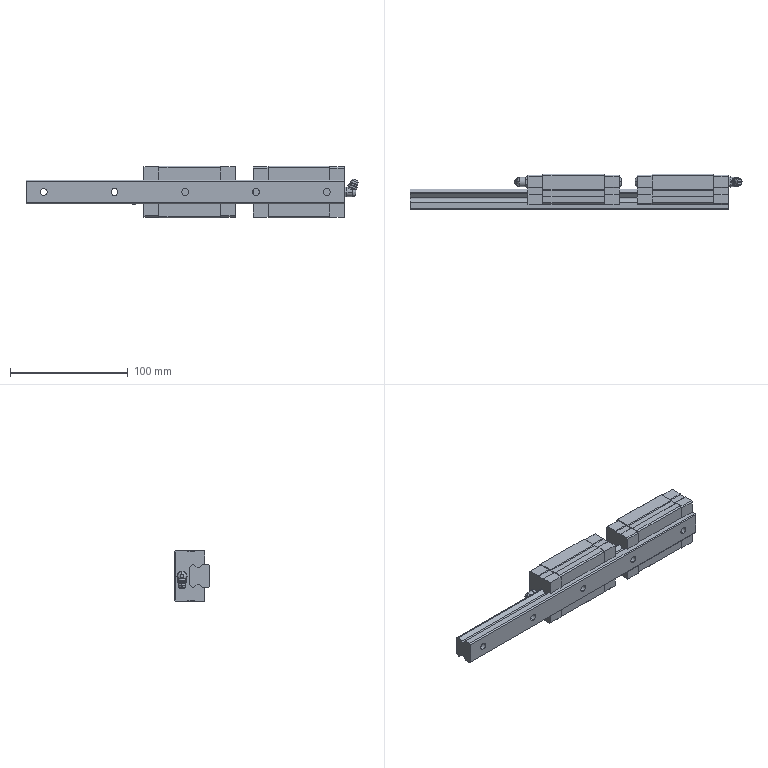Part | SolidWorks | 3 solids | 327 faces | box 281.473 x 30 x 44 mm | volume 214734 mm3 | plane 213 | cylinder 60 | cone 32 | spline 12 | torus 8 | sphere 2 | commonest cylinder face diameters 4.134 x16 5.8 x10 9.5 x10 7 x8 5.5 x4 6.6 x4